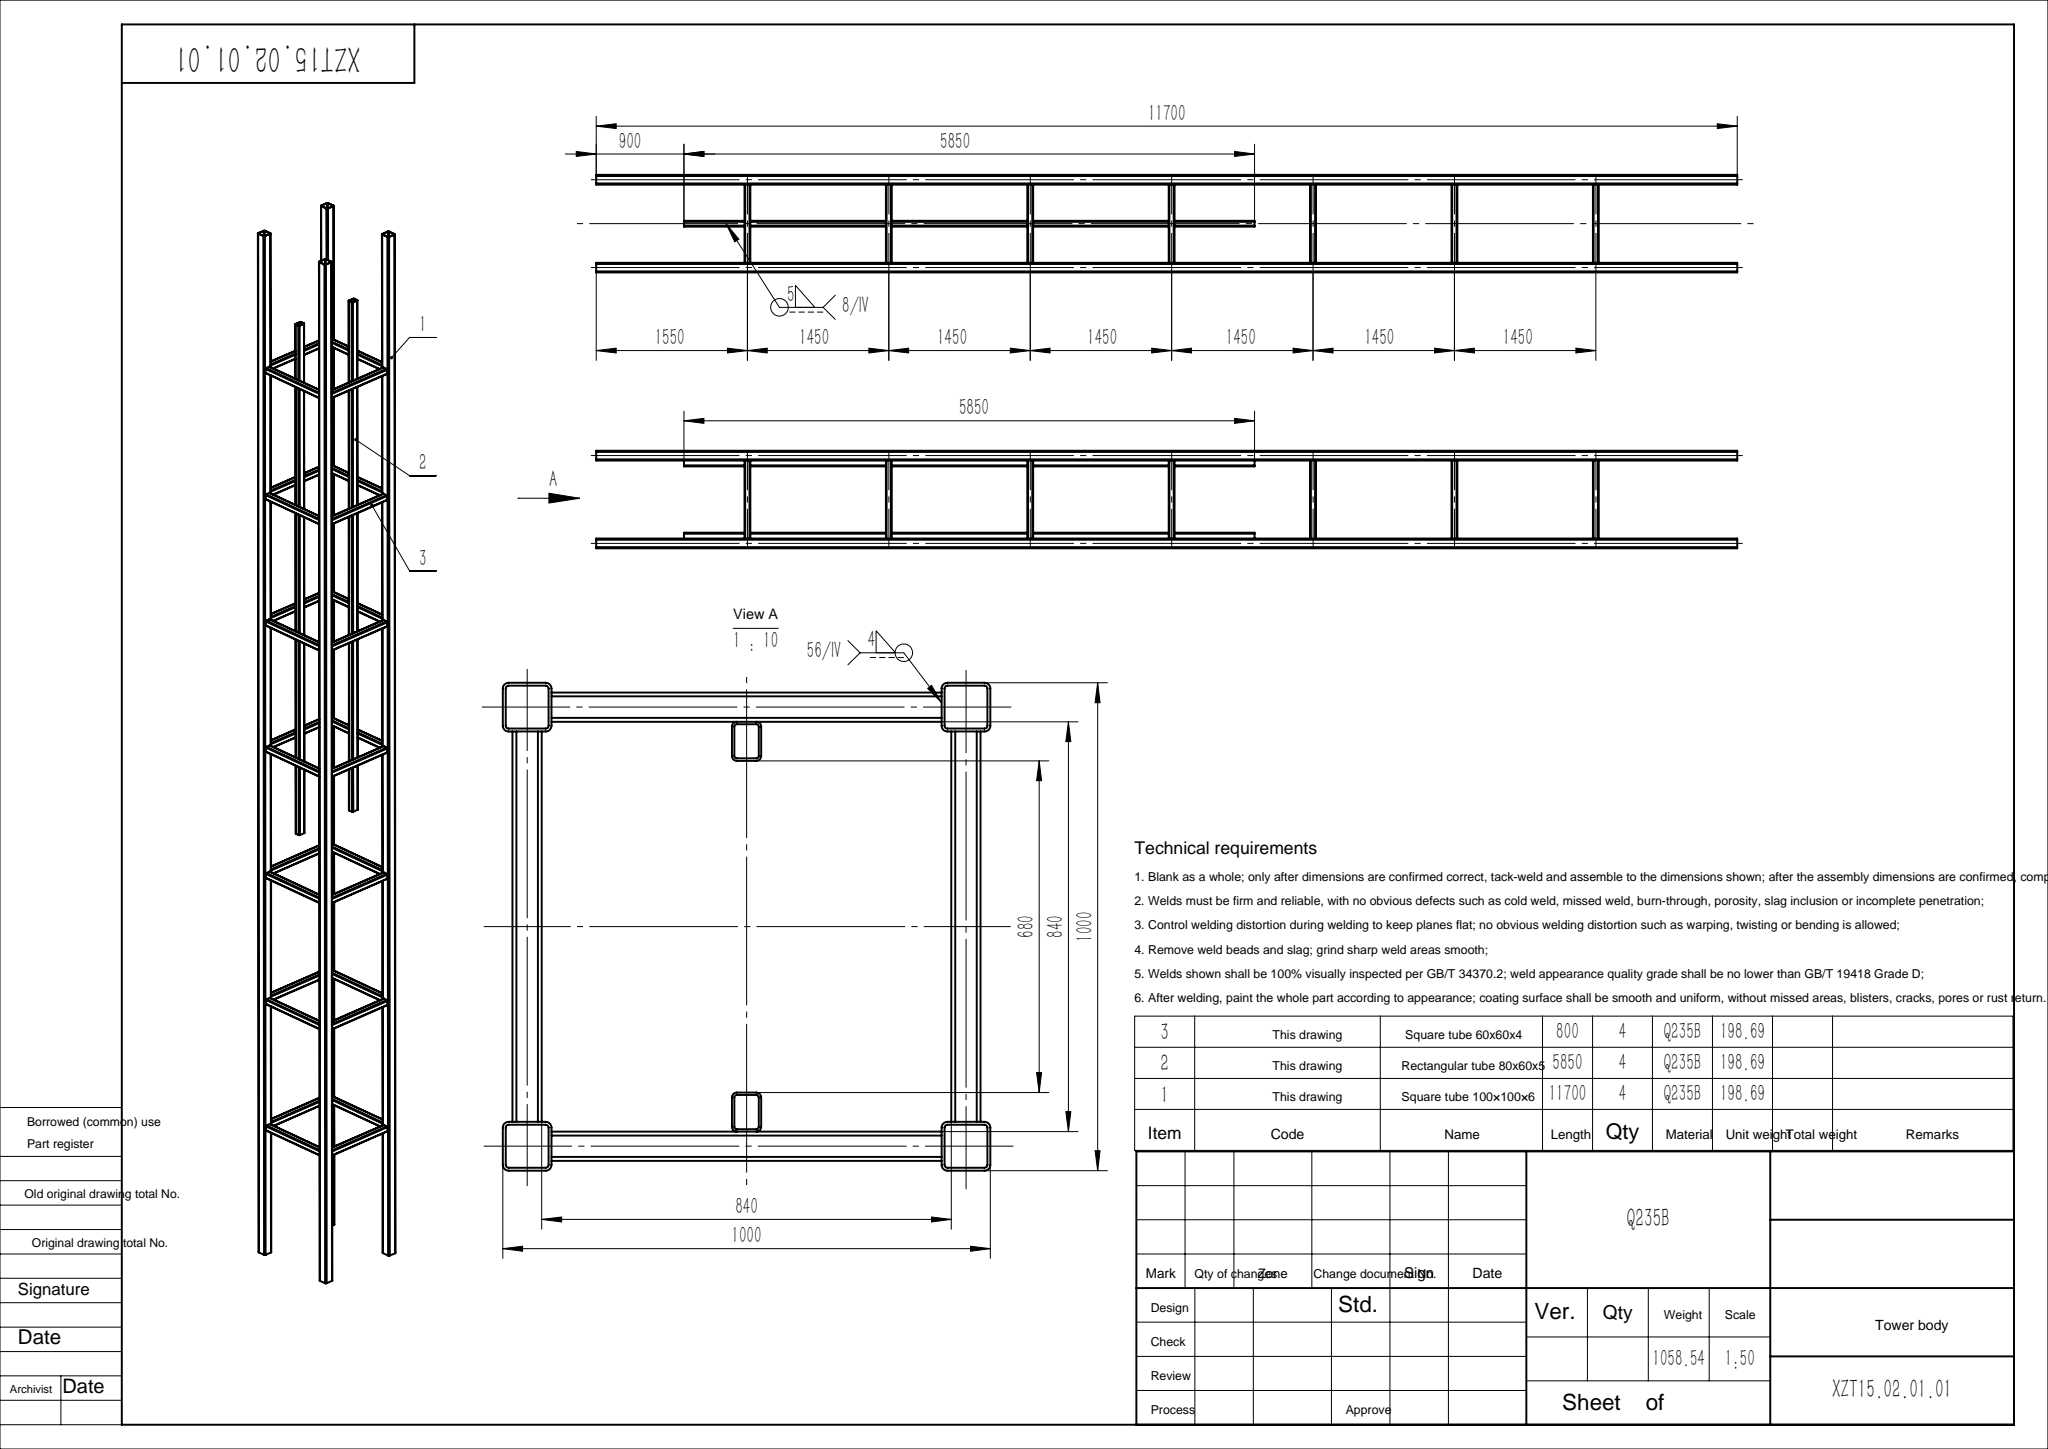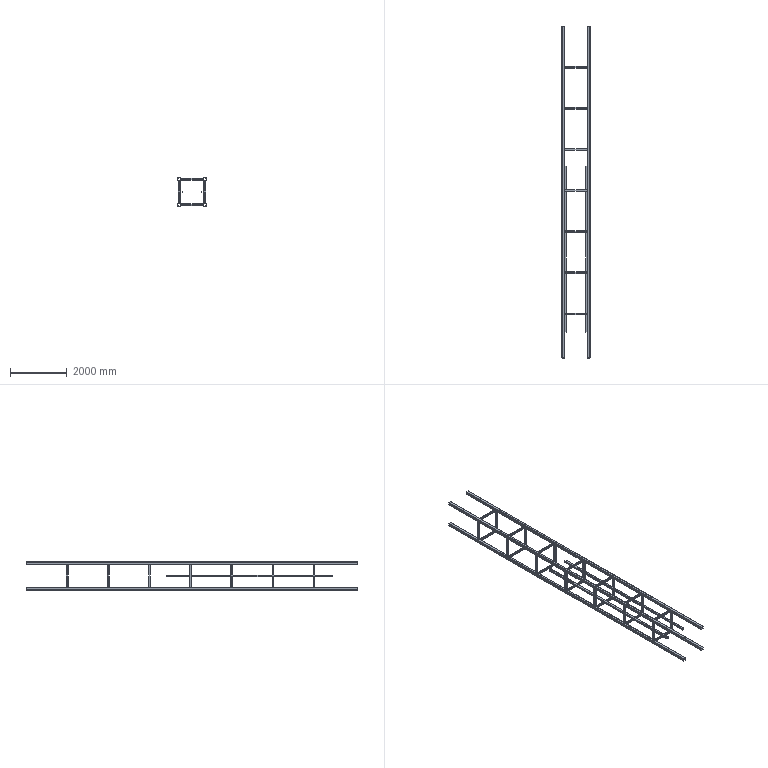Part | SolidWorks | features WeldMemberFeat 3, 3DProfileFeature 1, LPattern 1, WeldCornerFeat 1, WeldmentFeature 1 | 34 solids | 612 faces | box 1000 x 11700 x 1000 mm | volume 134846254 mm3 | plane 340 | cylinder 272 | commonest cylinder face diameters 8 x112 16 x112 12 x16 24 x16 10 x8 20 x8